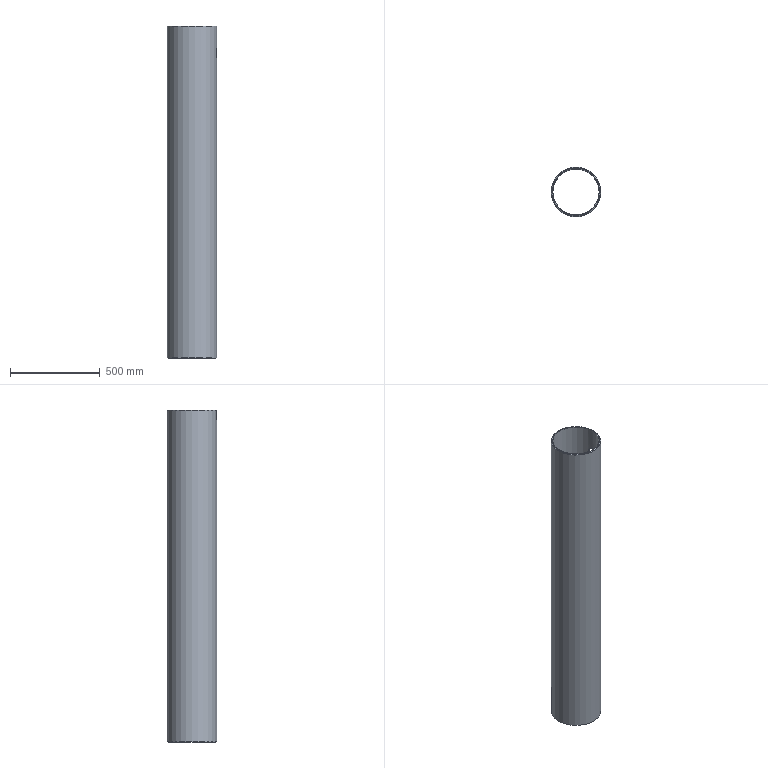Part | NX | features DATUM_CSYS 2, CHAMFER 1, CYLINDER 1, EXTRUDE 1, Resize Face 1, SHELL 1, SKETCH 1 | 1 solid | 7 faces | box 275 x 275 x 1849 mm | volume 12376930 mm3 | cylinder 3 | plane 2 | cone 2 | commonest cylinder face diameters 60 x1 259 x1 275 x1
STEP:
#1=CARTESIAN_POINT('',(137.5,0.,2.5));
#2=VERTEX_POINT('',#1);
#3=CARTESIAN_POINT('',(0.,0.,2.5));
#4=DIRECTION('',(0.,0.,1.));
#5=DIRECTION('',(1.,0.,0.));
#6=AXIS2_PLACEMENT_3D('',#3,#4,#5);
#7=CIRCLE('',#6,137.5);
#8=EDGE_CURVE('',#2,#2,#7,.T.);
#9=ORIENTED_EDGE('',*,*,#8,.T.);
#10=EDGE_LOOP('',(#9));
#11=FACE_BOUND('',#10,.T.);
#12=CARTESIAN_POINT('',(-137.5,0.,1846.7));
#13=VERTEX_POINT('',#12);
#14=CARTESIAN_POINT('',(0.,0.,1846.7));
#15=DIRECTION('',(0.,0.,-1.));
#16=DIRECTION('',(-1.,0.,0.));
#17=AXIS2_PLACEMENT_3D('',#14,#15,#16);
#18=CIRCLE('',#17,137.5);
#19=EDGE_CURVE('',#13,#13,#18,.T.);
#20=ORIENTED_EDGE('',*,*,#19,.T.);
#21=EDGE_LOOP('',(#20));
#22=FACE_BOUND('',#21,.T.);
#23=CARTESIAN_POINT('',(137.5,0.,1669.2));
#24=VERTEX_POINT('',#23);
#25=CARTESIAN_POINT('',(137.14,11.856,1670.791));
#26=CARTESIAN_POINT('',(137.679,-0.009269,1668.407));
#27=CARTESIAN_POINT('',(137.143,-11.819,1670.78));
#28=CARTESIAN_POINT('',(135.855,-21.765,1677.445));
#29=CARTESIAN_POINT('',(134.555,-28.42,1687.383));
#30=CARTESIAN_POINT('',(134.004,-30.786,1699.179));
#31=CARTESIAN_POINT('',(134.552,-28.435,1710.992));
#32=CARTESIAN_POINT('',(135.856,-21.764,1720.96));
#33=CARTESIAN_POINT('',(137.143,-11.813,1727.623));
#34=CARTESIAN_POINT('',(137.678,-0.01305,1729.986));
#35=CARTESIAN_POINT('',(137.145,11.791,1727.632));
#36=CARTESIAN_POINT('',(135.859,21.742,1720.978));
#37=CARTESIAN_POINT('',(134.556,28.414,1711.039));
#38=CARTESIAN_POINT('',(134.004,30.789,1699.218));
#39=CARTESIAN_POINT('',(134.553,28.431,1687.403));
#40=CARTESIAN_POINT('',(135.854,21.771,1677.455));
#41=CARTESIAN_POINT('',(137.14,11.856,1670.791));
#42=CARTESIAN_POINT('',(137.679,-0.009269,1668.407));
#43=CARTESIAN_POINT('',(137.143,-11.819,1670.78));
#44=B_SPLINE_CURVE_WITH_KNOTS('',3,(#25,#26,#27,#28,#29,#30,#31,#32,#33,#34,#35,#36,#37,#38,#39,#40,#41,#42,#43),.UNSPECIFIED.,.T.,.F.,(1,1,1,1,1,1,1,1,1,1,1,1,1,1,1,1,1,1,1,1,1,1,1),(-0.03527,-0.02352,-0.01176,0.,0.01176,0.02352,0.03527,0.04703,0.05879,0.07055,0.08231,0.09406,0.1058,0.1176,0.1293,0.1411,0.1529,0.1646,0.1764,0.1881,0.1999,0.2116,0.2234),.UNSPECIFIED.);
#45=EDGE_CURVE('',#24,#24,#44,.T.);
#46=ORIENTED_EDGE('',*,*,#45,.T.);
#47=EDGE_LOOP('',(#46));
#48=FACE_BOUND('',#47,.T.);
#49=CARTESIAN_POINT('',(0.,0.,0.));
#50=DIRECTION('',(0.,0.,1.));
#51=DIRECTION('',(1.,0.,0.));
#52=AXIS2_PLACEMENT_3D('',#49,#50,#51);
#53=CYLINDRICAL_SURFACE('',#52,137.5);
#54=ADVANCED_FACE('',(#11,#22,#48),#53,.T.);
#55=CARTESIAN_POINT('',(129.5,0.,1849.2));
#56=VERTEX_POINT('',#55);
#57=CARTESIAN_POINT('',(0.,0.,1849.2));
#58=DIRECTION('',(0.,0.,1.));
#59=DIRECTION('',(1.,0.,0.));
#60=AXIS2_PLACEMENT_3D('',#57,#58,#59);
#61=CIRCLE('',#60,129.5);
#62=EDGE_CURVE('',#56,#56,#61,.F.);
#63=ORIENTED_EDGE('',*,*,#62,.F.);
#64=EDGE_LOOP('',(#63));
#65=FACE_BOUND('',#64,.T.);
#66=CARTESIAN_POINT('',(-129.5,0.,0.));
#67=VERTEX_POINT('',#66);
#68=CARTESIAN_POINT('',(0.,0.,0.));
#69=DIRECTION('',(0.,0.,-1.));
#70=DIRECTION('',(-1.,0.,0.));
#71=AXIS2_PLACEMENT_3D('',#68,#69,#70);
#72=CIRCLE('',#71,129.5);
#73=EDGE_CURVE('',#67,#67,#72,.F.);
#74=ORIENTED_EDGE('',*,*,#73,.F.);
#75=EDGE_LOOP('',(#74));
#76=FACE_BOUND('',#75,.T.);
#77=CARTESIAN_POINT('',(129.5,0.,1669.2));
#78=VERTEX_POINT('',#77);
#79=CARTESIAN_POINT('',(129.118,11.859,1670.793));
#80=CARTESIAN_POINT('',(129.691,-0.008952,1668.406));
#81=CARTESIAN_POINT('',(129.12,-11.823,1670.781));
#82=CARTESIAN_POINT('',(127.753,-21.765,1677.446));
#83=CARTESIAN_POINT('',(126.369,-28.418,1687.379));
#84=CARTESIAN_POINT('',(125.782,-30.787,1699.178));
#85=CARTESIAN_POINT('',(126.366,-28.433,1710.996));
#86=CARTESIAN_POINT('',(127.754,-21.762,1720.961));
#87=CARTESIAN_POINT('',(129.121,-11.817,1727.621));
#88=CARTESIAN_POINT('',(129.689,-0.01338,1729.987));
#89=CARTESIAN_POINT('',(129.123,11.795,1727.631));
#90=CARTESIAN_POINT('',(127.757,21.743,1720.977));
#91=CARTESIAN_POINT('',(126.371,28.413,1711.042));
#92=CARTESIAN_POINT('',(125.781,30.79,1699.217));
#93=CARTESIAN_POINT('',(126.367,28.429,1687.398));
#94=CARTESIAN_POINT('',(127.751,21.77,1677.455));
#95=CARTESIAN_POINT('',(129.118,11.859,1670.793));
#96=CARTESIAN_POINT('',(129.691,-0.008952,1668.406));
#97=CARTESIAN_POINT('',(129.12,-11.823,1670.781));
#98=B_SPLINE_CURVE_WITH_KNOTS('',3,(#79,#80,#81,#82,#83,#84,#85,#86,#87,#88,#89,#90,#91,#92,#93,#94,#95,#96,#97),.UNSPECIFIED.,.T.,.F.,(1,1,1,1,1,1,1,1,1,1,1,1,1,1,1,1,1,1,1,1,1,1,1),(-0.03529,-0.02353,-0.01176,0.,0.01176,0.02353,0.03529,0.04705,0.05881,0.07058,0.08234,0.0941,0.1059,0.1176,0.1294,0.1412,0.1529,0.1647,0.1764,0.1882,0.2,0.2117,0.2235),.UNSPECIFIED.);
#99=EDGE_CURVE('',#78,#78,#98,.T.);
#100=ORIENTED_EDGE('',*,*,#99,.F.);
#101=EDGE_LOOP('',(#100));
#102=FACE_BOUND('',#101,.T.);
#103=CARTESIAN_POINT('',(0.,0.,0.));
#104=DIRECTION('',(0.,0.,1.));
#105=DIRECTION('',(1.,0.,0.));
#106=AXIS2_PLACEMENT_3D('',#103,#104,#105);
#107=CYLINDRICAL_SURFACE('',#106,129.5);
#108=ADVANCED_FACE('',(#65,#76,#102),#107,.F.);
#109=CARTESIAN_POINT('',(133.17,0.,1849.2));
#110=VERTEX_POINT('',#109);
#111=CARTESIAN_POINT('',(0.,0.,1849.2));
#112=DIRECTION('',(0.,0.,1.));
#113=DIRECTION('',(1.,0.,0.));
#114=AXIS2_PLACEMENT_3D('',#111,#112,#113);
#115=CIRCLE('',#114,133.17);
#116=EDGE_CURVE('',#110,#110,#115,.T.);
#117=ORIENTED_EDGE('',*,*,#116,.T.);
#118=EDGE_LOOP('',(#117));
#119=FACE_BOUND('',#118,.T.);
#120=ORIENTED_EDGE('',*,*,#62,.T.);
#121=EDGE_LOOP('',(#120));
#122=FACE_BOUND('',#121,.T.);
#123=CARTESIAN_POINT('',(0.,0.,1849.2));
#124=DIRECTION('',(0.,0.,1.));
#125=DIRECTION('',(1.,0.,0.));
#126=AXIS2_PLACEMENT_3D('',#123,#124,#125);
#127=PLANE('',#126);
#128=ADVANCED_FACE('',(#119,#122),#127,.T.);
#129=CARTESIAN_POINT('',(-133.17,0.,0.));
#130=VERTEX_POINT('',#129);
#131=CARTESIAN_POINT('',(0.,0.,0.));
#132=DIRECTION('',(0.,0.,-1.));
#133=DIRECTION('',(-1.,0.,0.));
#134=AXIS2_PLACEMENT_3D('',#131,#132,#133);
#135=CIRCLE('',#134,133.17);
#136=EDGE_CURVE('',#130,#130,#135,.T.);
#137=ORIENTED_EDGE('',*,*,#136,.T.);
#138=EDGE_LOOP('',(#137));
#139=FACE_BOUND('',#138,.T.);
#140=ORIENTED_EDGE('',*,*,#73,.T.);
#141=EDGE_LOOP('',(#140));
#142=FACE_BOUND('',#141,.T.);
#143=CARTESIAN_POINT('',(0.,0.,0.));
#144=DIRECTION('',(0.,0.,-1.));
#145=DIRECTION('',(-1.,0.,0.));
#146=AXIS2_PLACEMENT_3D('',#143,#144,#145);
#147=PLANE('',#146);
#148=ADVANCED_FACE('',(#139,#142),#147,.T.);
#149=ORIENTED_EDGE('',*,*,#116,.F.);
#150=EDGE_LOOP('',(#149));
#151=FACE_BOUND('',#150,.T.);
#152=ORIENTED_EDGE('',*,*,#19,.F.);
#153=EDGE_LOOP('',(#152));
#154=FACE_BOUND('',#153,.T.);
#155=CARTESIAN_POINT('',(0.,0.,1846.7));
#156=DIRECTION('',(0.,0.,-1.));
#157=DIRECTION('',(-1.,0.,0.));
#158=AXIS2_PLACEMENT_3D('',#155,#156,#157);
#159=CONICAL_SURFACE('',#158,137.5,1.047);
#160=ADVANCED_FACE('',(#151,#154),#159,.T.);
#161=ORIENTED_EDGE('',*,*,#136,.F.);
#162=EDGE_LOOP('',(#161));
#163=FACE_BOUND('',#162,.T.);
#164=ORIENTED_EDGE('',*,*,#8,.F.);
#165=EDGE_LOOP('',(#164));
#166=FACE_BOUND('',#165,.T.);
#167=CARTESIAN_POINT('',(0.,0.,2.5));
#168=DIRECTION('',(0.,0.,1.));
#169=DIRECTION('',(1.,0.,0.));
#170=AXIS2_PLACEMENT_3D('',#167,#168,#169);
#171=CONICAL_SURFACE('',#170,137.5,1.047);
#172=ADVANCED_FACE('',(#163,#166),#171,.T.);
#173=ORIENTED_EDGE('',*,*,#45,.F.);
#174=EDGE_LOOP('',(#173));
#175=FACE_BOUND('',#174,.T.);
#176=ORIENTED_EDGE('',*,*,#99,.T.);
#177=EDGE_LOOP('',(#176));
#178=FACE_BOUND('',#177,.T.);
#179=CARTESIAN_POINT('',(720.,0.,1699.2));
#180=DIRECTION('',(-1.,0.,0.));
#181=DIRECTION('',(0.,0.,1.));
#182=AXIS2_PLACEMENT_3D('',#179,#180,#181);
#183=CYLINDRICAL_SURFACE('',#182,30.);
#184=ADVANCED_FACE('',(#175,#178),#183,.F.);
#185=CLOSED_SHELL('',(#54,#108,#128,#148,#160,#172,#184));
#186=MANIFOLD_SOLID_BREP('',#185);
#187=(LENGTH_UNIT()NAMED_UNIT(*)SI_UNIT(.MILLI.,.METRE.));
#188=UNCERTAINTY_MEASURE_WITH_UNIT(LENGTH_MEASURE(0.0508),#187,'','');
#189=(NAMED_UNIT(*)PLANE_ANGLE_UNIT()SI_UNIT($,.RADIAN.));
#190=(NAMED_UNIT(*)SI_UNIT($,.STERADIAN.)SOLID_ANGLE_UNIT());
#191=(GEOMETRIC_REPRESENTATION_CONTEXT(3)GLOBAL_UNCERTAINTY_ASSIGNED_CONTEXT((#188))GLOBAL_UNIT_ASSIGNED_CONTEXT((#187,#189,#190))REPRESENTATION_CONTEXT('',''));
#192=ADVANCED_BREP_SHAPE_REPRESENTATION('',(#186),#191);